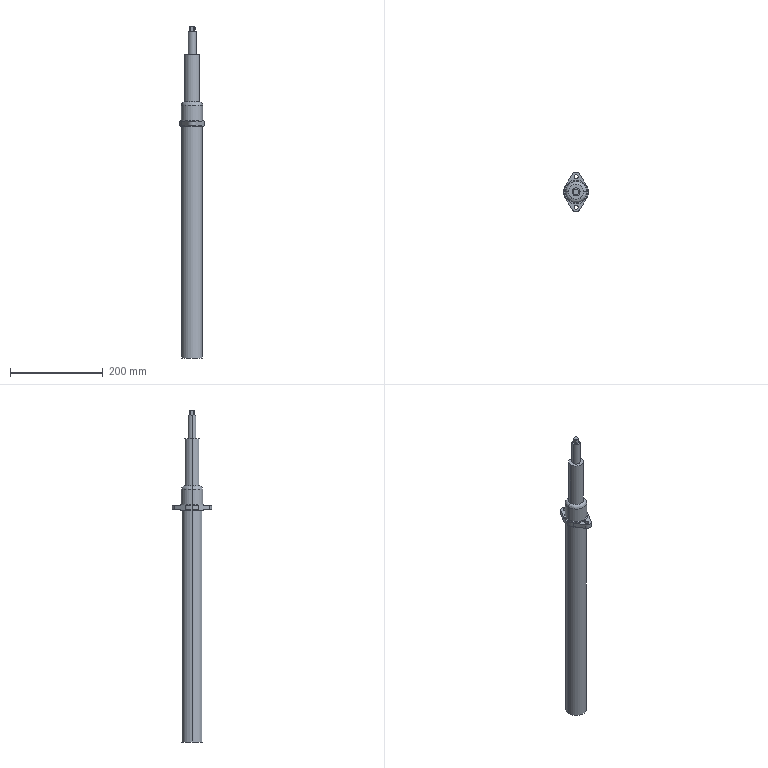Part | STEP file | 35N torque tester | 1 solid | 48 faces | box 54 x 85 x 717 mm | volume 972742 mm3 | cylinder 23 | plane 21 | spline 4 | commonest cylinder face diameters 8.8 x4 51 x4 54 x3 3 x2 17.4 x2 19 x2